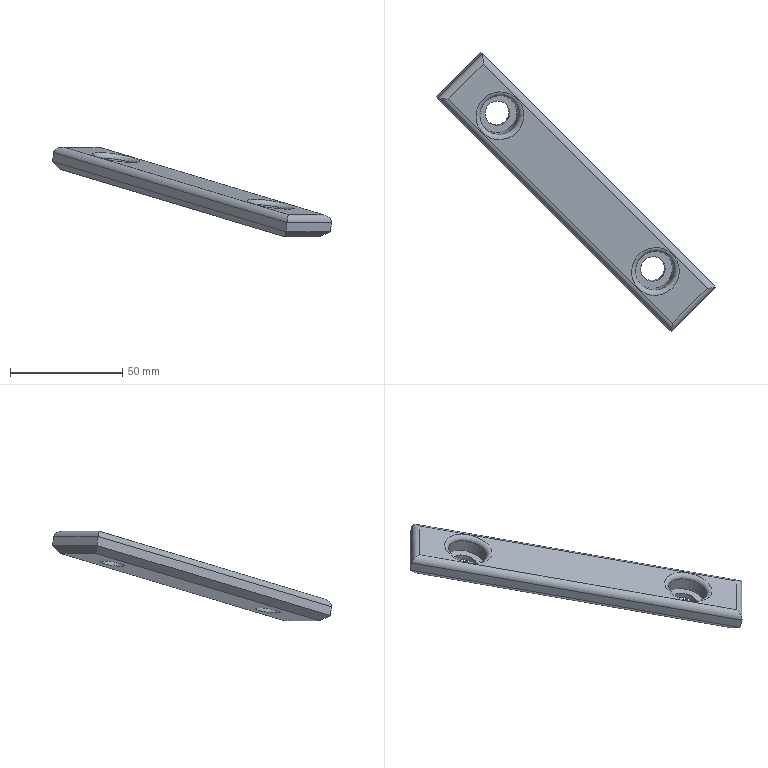Part | STEP file | gslz 2016.10.28-13_id1558_x_t | 1 solid | 151 faces | box 124.158 x 124.158 x 39.786 mm | volume 35566 mm3 | plane 102 | other 39 | cylinder 8 | torus 2 | commonest cylinder face diameters 6 x4 11 x2 17.5 x2